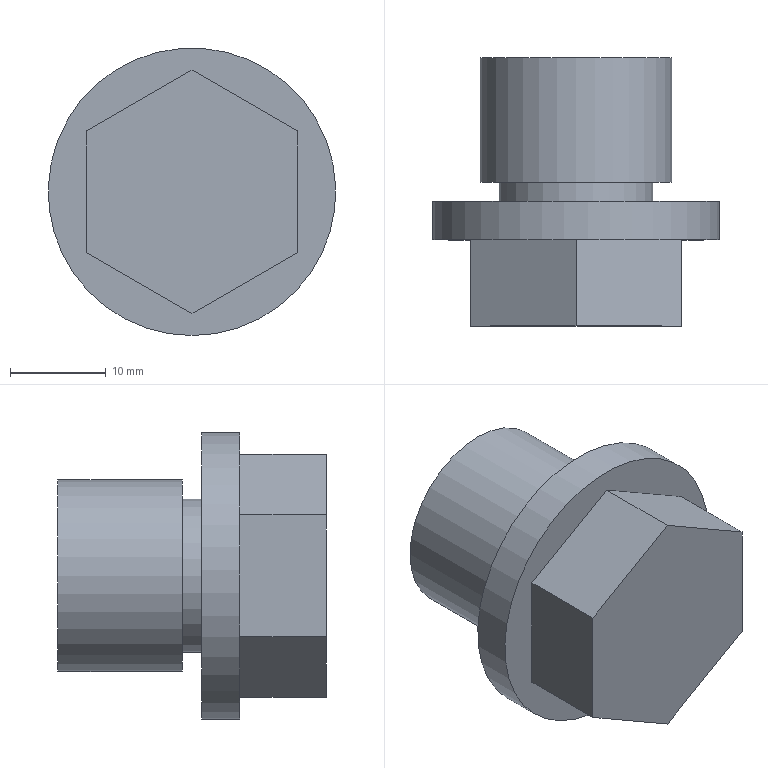Part | NX | features DATUM_CSYS 3, SKETCH 2, EXTRUDE 1, SWP104 1, SYMBOLIC_THREAD 1 | 1 solid | 14 faces | box 30 x 28 x 30 mm | volume 11086 mm3 | plane 11 | cylinder 3 | commonest cylinder face diameters 16 x1 20 x1 30 x1
STEP:
#1=CARTESIAN_POINT('',(-11.,0.,6.351));
#2=VERTEX_POINT('',#1);
#3=CARTESIAN_POINT('',(-11.,0.,-6.351));
#4=VERTEX_POINT('',#3);
#5=CARTESIAN_POINT('',(-11.,0.,6.351));
#6=DIRECTION('',(0.,0.,-1.));
#7=VECTOR('',#6,1000.);
#8=LINE('',#5,#7);
#9=EDGE_CURVE('',#2,#4,#8,.T.);
#10=ORIENTED_EDGE('',*,*,#9,.T.);
#11=CARTESIAN_POINT('',(-11.,-9.,-6.351));
#12=VERTEX_POINT('',#11);
#13=CARTESIAN_POINT('',(-11.,-9.,-6.351));
#14=DIRECTION('',(0.,1.,0.));
#15=VECTOR('',#14,1000.);
#16=LINE('',#13,#15);
#17=EDGE_CURVE('',#12,#4,#16,.T.);
#18=ORIENTED_EDGE('',*,*,#17,.F.);
#19=CARTESIAN_POINT('',(-11.,-9.,6.351));
#20=VERTEX_POINT('',#19);
#21=CARTESIAN_POINT('',(-11.,-9.,6.351));
#22=DIRECTION('',(0.,0.,-1.));
#23=VECTOR('',#22,1000.);
#24=LINE('',#21,#23);
#25=EDGE_CURVE('',#20,#12,#24,.T.);
#26=ORIENTED_EDGE('',*,*,#25,.F.);
#27=CARTESIAN_POINT('',(-11.,-9.,6.351));
#28=DIRECTION('',(0.,1.,0.));
#29=VECTOR('',#28,1000.);
#30=LINE('',#27,#29);
#31=EDGE_CURVE('',#20,#2,#30,.T.);
#32=ORIENTED_EDGE('',*,*,#31,.T.);
#33=EDGE_LOOP('',(#10,#18,#26,#32));
#34=FACE_BOUND('',#33,.T.);
#35=CARTESIAN_POINT('',(-11.,-9.,6.351));
#36=DIRECTION('',(1.,0.,0.));
#37=DIRECTION('',(0.,0.,-1.));
#38=AXIS2_PLACEMENT_3D('',#35,#36,#37);
#39=PLANE('',#38);
#40=ADVANCED_FACE('',(#34),#39,.F.);
#41=CARTESIAN_POINT('',(0.,0.,-12.702));
#42=VERTEX_POINT('',#41);
#43=CARTESIAN_POINT('',(-11.,0.,-6.351));
#44=DIRECTION('',(0.866,0.,-0.5));
#45=VECTOR('',#44,1000.);
#46=LINE('',#43,#45);
#47=EDGE_CURVE('',#4,#42,#46,.T.);
#48=ORIENTED_EDGE('',*,*,#47,.T.);
#49=CARTESIAN_POINT('',(0.,-9.,-12.702));
#50=VERTEX_POINT('',#49);
#51=CARTESIAN_POINT('',(0.,-9.,-12.702));
#52=DIRECTION('',(0.,1.,0.));
#53=VECTOR('',#52,1000.);
#54=LINE('',#51,#53);
#55=EDGE_CURVE('',#50,#42,#54,.T.);
#56=ORIENTED_EDGE('',*,*,#55,.F.);
#57=CARTESIAN_POINT('',(-11.,-9.,-6.351));
#58=DIRECTION('',(0.866,0.,-0.5));
#59=VECTOR('',#58,1000.);
#60=LINE('',#57,#59);
#61=EDGE_CURVE('',#12,#50,#60,.T.);
#62=ORIENTED_EDGE('',*,*,#61,.F.);
#63=ORIENTED_EDGE('',*,*,#17,.T.);
#64=EDGE_LOOP('',(#48,#56,#62,#63));
#65=FACE_BOUND('',#64,.T.);
#66=CARTESIAN_POINT('',(-11.,-9.,-6.351));
#67=DIRECTION('',(0.5,0.,0.866));
#68=DIRECTION('',(0.866,0.,-0.5));
#69=AXIS2_PLACEMENT_3D('',#66,#67,#68);
#70=PLANE('',#69);
#71=ADVANCED_FACE('',(#65),#70,.F.);
#72=CARTESIAN_POINT('',(11.,0.,-6.351));
#73=VERTEX_POINT('',#72);
#74=CARTESIAN_POINT('',(0.,0.,-12.702));
#75=DIRECTION('',(0.866,0.,0.5));
#76=VECTOR('',#75,1000.);
#77=LINE('',#74,#76);
#78=EDGE_CURVE('',#42,#73,#77,.T.);
#79=ORIENTED_EDGE('',*,*,#78,.T.);
#80=CARTESIAN_POINT('',(11.,-9.,-6.351));
#81=VERTEX_POINT('',#80);
#82=CARTESIAN_POINT('',(11.,-9.,-6.351));
#83=DIRECTION('',(0.,1.,0.));
#84=VECTOR('',#83,1000.);
#85=LINE('',#82,#84);
#86=EDGE_CURVE('',#81,#73,#85,.T.);
#87=ORIENTED_EDGE('',*,*,#86,.F.);
#88=CARTESIAN_POINT('',(0.,-9.,-12.702));
#89=DIRECTION('',(0.866,0.,0.5));
#90=VECTOR('',#89,1000.);
#91=LINE('',#88,#90);
#92=EDGE_CURVE('',#50,#81,#91,.T.);
#93=ORIENTED_EDGE('',*,*,#92,.F.);
#94=ORIENTED_EDGE('',*,*,#55,.T.);
#95=EDGE_LOOP('',(#79,#87,#93,#94));
#96=FACE_BOUND('',#95,.T.);
#97=CARTESIAN_POINT('',(0.,-9.,-12.702));
#98=DIRECTION('',(-0.5,0.,0.866));
#99=DIRECTION('',(0.866,0.,0.5));
#100=AXIS2_PLACEMENT_3D('',#97,#98,#99);
#101=PLANE('',#100);
#102=ADVANCED_FACE('',(#96),#101,.F.);
#103=CARTESIAN_POINT('',(11.,0.,6.351));
#104=VERTEX_POINT('',#103);
#105=CARTESIAN_POINT('',(11.,0.,-6.351));
#106=DIRECTION('',(0.,0.,1.));
#107=VECTOR('',#106,1000.);
#108=LINE('',#105,#107);
#109=EDGE_CURVE('',#73,#104,#108,.T.);
#110=ORIENTED_EDGE('',*,*,#109,.T.);
#111=CARTESIAN_POINT('',(11.,-9.,6.351));
#112=VERTEX_POINT('',#111);
#113=CARTESIAN_POINT('',(11.,-9.,6.351));
#114=DIRECTION('',(0.,1.,0.));
#115=VECTOR('',#114,1000.);
#116=LINE('',#113,#115);
#117=EDGE_CURVE('',#112,#104,#116,.T.);
#118=ORIENTED_EDGE('',*,*,#117,.F.);
#119=CARTESIAN_POINT('',(11.,-9.,-6.351));
#120=DIRECTION('',(0.,0.,1.));
#121=VECTOR('',#120,1000.);
#122=LINE('',#119,#121);
#123=EDGE_CURVE('',#81,#112,#122,.T.);
#124=ORIENTED_EDGE('',*,*,#123,.F.);
#125=ORIENTED_EDGE('',*,*,#86,.T.);
#126=EDGE_LOOP('',(#110,#118,#124,#125));
#127=FACE_BOUND('',#126,.T.);
#128=CARTESIAN_POINT('',(11.,-9.,-6.351));
#129=DIRECTION('',(-1.,0.,0.));
#130=DIRECTION('',(0.,0.,1.));
#131=AXIS2_PLACEMENT_3D('',#128,#129,#130);
#132=PLANE('',#131);
#133=ADVANCED_FACE('',(#127),#132,.F.);
#134=CARTESIAN_POINT('',(0.,0.,12.702));
#135=VERTEX_POINT('',#134);
#136=CARTESIAN_POINT('',(11.,0.,6.351));
#137=DIRECTION('',(-0.866,0.,0.5));
#138=VECTOR('',#137,1000.);
#139=LINE('',#136,#138);
#140=EDGE_CURVE('',#104,#135,#139,.T.);
#141=ORIENTED_EDGE('',*,*,#140,.T.);
#142=CARTESIAN_POINT('',(0.,-9.,12.702));
#143=VERTEX_POINT('',#142);
#144=CARTESIAN_POINT('',(0.,-9.,12.702));
#145=DIRECTION('',(0.,1.,0.));
#146=VECTOR('',#145,1000.);
#147=LINE('',#144,#146);
#148=EDGE_CURVE('',#143,#135,#147,.T.);
#149=ORIENTED_EDGE('',*,*,#148,.F.);
#150=CARTESIAN_POINT('',(11.,-9.,6.351));
#151=DIRECTION('',(-0.866,0.,0.5));
#152=VECTOR('',#151,1000.);
#153=LINE('',#150,#152);
#154=EDGE_CURVE('',#112,#143,#153,.T.);
#155=ORIENTED_EDGE('',*,*,#154,.F.);
#156=ORIENTED_EDGE('',*,*,#117,.T.);
#157=EDGE_LOOP('',(#141,#149,#155,#156));
#158=FACE_BOUND('',#157,.T.);
#159=CARTESIAN_POINT('',(11.,-9.,6.351));
#160=DIRECTION('',(-0.5,0.,-0.866));
#161=DIRECTION('',(-0.866,0.,0.5));
#162=AXIS2_PLACEMENT_3D('',#159,#160,#161);
#163=PLANE('',#162);
#164=ADVANCED_FACE('',(#158),#163,.F.);
#165=CARTESIAN_POINT('',(0.,0.,12.702));
#166=DIRECTION('',(-0.866,0.,-0.5));
#167=VECTOR('',#166,1000.);
#168=LINE('',#165,#167);
#169=EDGE_CURVE('',#135,#2,#168,.T.);
#170=ORIENTED_EDGE('',*,*,#169,.T.);
#171=ORIENTED_EDGE('',*,*,#31,.F.);
#172=CARTESIAN_POINT('',(0.,-9.,12.702));
#173=DIRECTION('',(-0.866,0.,-0.5));
#174=VECTOR('',#173,1000.);
#175=LINE('',#172,#174);
#176=EDGE_CURVE('',#143,#20,#175,.T.);
#177=ORIENTED_EDGE('',*,*,#176,.F.);
#178=ORIENTED_EDGE('',*,*,#148,.T.);
#179=EDGE_LOOP('',(#170,#171,#177,#178));
#180=FACE_BOUND('',#179,.T.);
#181=CARTESIAN_POINT('',(0.,-9.,12.702));
#182=DIRECTION('',(0.5,0.,-0.866));
#183=DIRECTION('',(-0.866,0.,-0.5));
#184=AXIS2_PLACEMENT_3D('',#181,#182,#183);
#185=PLANE('',#184);
#186=ADVANCED_FACE('',(#180),#185,.F.);
#187=ORIENTED_EDGE('',*,*,#25,.T.);
#188=ORIENTED_EDGE('',*,*,#61,.T.);
#189=ORIENTED_EDGE('',*,*,#92,.T.);
#190=ORIENTED_EDGE('',*,*,#123,.T.);
#191=ORIENTED_EDGE('',*,*,#154,.T.);
#192=ORIENTED_EDGE('',*,*,#176,.T.);
#193=EDGE_LOOP('',(#187,#188,#189,#190,#191,#192));
#194=FACE_BOUND('',#193,.T.);
#195=CARTESIAN_POINT('',(0.,-9.,0.));
#196=DIRECTION('',(0.,-1.,0.));
#197=DIRECTION('',(0.,0.,-1.));
#198=AXIS2_PLACEMENT_3D('',#195,#196,#197);
#199=PLANE('',#198);
#200=ADVANCED_FACE('',(#194),#199,.T.);
#201=ORIENTED_EDGE('',*,*,#9,.F.);
#202=ORIENTED_EDGE('',*,*,#169,.F.);
#203=ORIENTED_EDGE('',*,*,#140,.F.);
#204=ORIENTED_EDGE('',*,*,#109,.F.);
#205=ORIENTED_EDGE('',*,*,#78,.F.);
#206=ORIENTED_EDGE('',*,*,#47,.F.);
#207=EDGE_LOOP('',(#201,#202,#203,#204,#205,#206));
#208=FACE_BOUND('',#207,.T.);
#209=CARTESIAN_POINT('',(0.,0.,-15.));
#210=VERTEX_POINT('',#209);
#211=CARTESIAN_POINT('',(0.,0.,0.));
#212=DIRECTION('',(0.,-1.,0.));
#213=DIRECTION('',(0.,0.,-1.));
#214=AXIS2_PLACEMENT_3D('',#211,#212,#213);
#215=CIRCLE('',#214,15.);
#216=EDGE_CURVE('',#210,#210,#215,.T.);
#217=ORIENTED_EDGE('',*,*,#216,.T.);
#218=EDGE_LOOP('',(#217));
#219=FACE_BOUND('',#218,.T.);
#220=CARTESIAN_POINT('',(0.,0.,15.));
#221=DIRECTION('',(0.,1.,0.));
#222=DIRECTION('',(0.,0.,1.));
#223=AXIS2_PLACEMENT_3D('',#220,#221,#222);
#224=PLANE('',#223);
#225=ADVANCED_FACE('',(#208,#219),#224,.F.);
#226=CARTESIAN_POINT('',(0.,19.,-10.));
#227=VERTEX_POINT('',#226);
#228=CARTESIAN_POINT('',(0.,19.,0.));
#229=DIRECTION('',(0.,-1.,0.));
#230=DIRECTION('',(0.,0.,-1.));
#231=AXIS2_PLACEMENT_3D('',#228,#229,#230);
#232=CIRCLE('',#231,10.);
#233=EDGE_CURVE('',#227,#227,#232,.T.);
#234=ORIENTED_EDGE('',*,*,#233,.F.);
#235=EDGE_LOOP('',(#234));
#236=FACE_BOUND('',#235,.T.);
#237=CARTESIAN_POINT('',(0.,19.,0.));
#238=DIRECTION('',(0.,-1.,0.));
#239=DIRECTION('',(0.,0.,-1.));
#240=AXIS2_PLACEMENT_3D('',#237,#238,#239);
#241=PLANE('',#240);
#242=ADVANCED_FACE('',(#236),#241,.F.);
#243=CARTESIAN_POINT('',(0.,6.,-10.));
#244=VERTEX_POINT('',#243);
#245=CARTESIAN_POINT('',(0.,6.,0.));
#246=DIRECTION('',(0.,-1.,0.));
#247=DIRECTION('',(0.,0.,-1.));
#248=AXIS2_PLACEMENT_3D('',#245,#246,#247);
#249=CIRCLE('',#248,10.);
#250=EDGE_CURVE('',#244,#244,#249,.T.);
#251=ORIENTED_EDGE('',*,*,#250,.F.);
#252=EDGE_LOOP('',(#251));
#253=FACE_BOUND('',#252,.T.);
#254=ORIENTED_EDGE('',*,*,#233,.T.);
#255=EDGE_LOOP('',(#254));
#256=FACE_BOUND('',#255,.T.);
#257=CARTESIAN_POINT('',(0.,19.,0.));
#258=DIRECTION('',(0.,-1.,0.));
#259=DIRECTION('',(0.,0.,-1.));
#260=AXIS2_PLACEMENT_3D('',#257,#258,#259);
#261=CYLINDRICAL_SURFACE('',#260,10.);
#262=ADVANCED_FACE('',(#253,#256),#261,.T.);
#263=CARTESIAN_POINT('',(0.,6.,-8.));
#264=VERTEX_POINT('',#263);
#265=CARTESIAN_POINT('',(0.,6.,0.));
#266=DIRECTION('',(0.,-1.,0.));
#267=DIRECTION('',(0.,0.,-1.));
#268=AXIS2_PLACEMENT_3D('',#265,#266,#267);
#269=CIRCLE('',#268,8.);
#270=EDGE_CURVE('',#264,#264,#269,.T.);
#271=ORIENTED_EDGE('',*,*,#270,.F.);
#272=EDGE_LOOP('',(#271));
#273=FACE_BOUND('',#272,.T.);
#274=ORIENTED_EDGE('',*,*,#250,.T.);
#275=EDGE_LOOP('',(#274));
#276=FACE_BOUND('',#275,.T.);
#277=CARTESIAN_POINT('',(0.,6.,10.));
#278=DIRECTION('',(0.,1.,0.));
#279=DIRECTION('',(0.,0.,1.));
#280=AXIS2_PLACEMENT_3D('',#277,#278,#279);
#281=PLANE('',#280);
#282=ADVANCED_FACE('',(#273,#276),#281,.F.);
#283=CARTESIAN_POINT('',(0.,4.,-8.));
#284=VERTEX_POINT('',#283);
#285=CARTESIAN_POINT('',(0.,4.,0.));
#286=DIRECTION('',(0.,-1.,0.));
#287=DIRECTION('',(0.,0.,-1.));
#288=AXIS2_PLACEMENT_3D('',#285,#286,#287);
#289=CIRCLE('',#288,8.);
#290=EDGE_CURVE('',#284,#284,#289,.T.);
#291=ORIENTED_EDGE('',*,*,#290,.F.);
#292=EDGE_LOOP('',(#291));
#293=FACE_BOUND('',#292,.T.);
#294=ORIENTED_EDGE('',*,*,#270,.T.);
#295=EDGE_LOOP('',(#294));
#296=FACE_BOUND('',#295,.T.);
#297=CARTESIAN_POINT('',(0.,19.,0.));
#298=DIRECTION('',(0.,-1.,0.));
#299=DIRECTION('',(0.,0.,-1.));
#300=AXIS2_PLACEMENT_3D('',#297,#298,#299);
#301=CYLINDRICAL_SURFACE('',#300,8.);
#302=ADVANCED_FACE('',(#293,#296),#301,.T.);
#303=CARTESIAN_POINT('',(0.,4.,-15.));
#304=VERTEX_POINT('',#303);
#305=CARTESIAN_POINT('',(0.,4.,0.));
#306=DIRECTION('',(0.,-1.,0.));
#307=DIRECTION('',(0.,0.,-1.));
#308=AXIS2_PLACEMENT_3D('',#305,#306,#307);
#309=CIRCLE('',#308,15.);
#310=EDGE_CURVE('',#304,#304,#309,.T.);
#311=ORIENTED_EDGE('',*,*,#310,.F.);
#312=EDGE_LOOP('',(#311));
#313=FACE_BOUND('',#312,.T.);
#314=ORIENTED_EDGE('',*,*,#290,.T.);
#315=EDGE_LOOP('',(#314));
#316=FACE_BOUND('',#315,.T.);
#317=CARTESIAN_POINT('',(0.,4.,8.));
#318=DIRECTION('',(0.,-1.,0.));
#319=DIRECTION('',(0.,0.,-1.));
#320=AXIS2_PLACEMENT_3D('',#317,#318,#319);
#321=PLANE('',#320);
#322=ADVANCED_FACE('',(#313,#316),#321,.F.);
#323=ORIENTED_EDGE('',*,*,#216,.F.);
#324=EDGE_LOOP('',(#323));
#325=FACE_BOUND('',#324,.T.);
#326=ORIENTED_EDGE('',*,*,#310,.T.);
#327=EDGE_LOOP('',(#326));
#328=FACE_BOUND('',#327,.T.);
#329=CARTESIAN_POINT('',(0.,19.,0.));
#330=DIRECTION('',(0.,-1.,0.));
#331=DIRECTION('',(0.,0.,-1.));
#332=AXIS2_PLACEMENT_3D('',#329,#330,#331);
#333=CYLINDRICAL_SURFACE('',#332,15.);
#334=ADVANCED_FACE('',(#325,#328),#333,.T.);
#335=CLOSED_SHELL('',(#40,#71,#102,#133,#164,#186,#200,#225,#242,#262,#282,#302,#322,#334));
#336=MANIFOLD_SOLID_BREP('',#335);
#337=(LENGTH_UNIT()NAMED_UNIT(*)SI_UNIT(.MILLI.,.METRE.));
#338=UNCERTAINTY_MEASURE_WITH_UNIT(LENGTH_MEASURE(0.00001),#337,'','');
#339=(NAMED_UNIT(*)PLANE_ANGLE_UNIT()SI_UNIT($,.RADIAN.));
#340=(NAMED_UNIT(*)SI_UNIT($,.STERADIAN.)SOLID_ANGLE_UNIT());
#341=(GEOMETRIC_REPRESENTATION_CONTEXT(3)GLOBAL_UNCERTAINTY_ASSIGNED_CONTEXT((#338))GLOBAL_UNIT_ASSIGNED_CONTEXT((#337,#339,#340))REPRESENTATION_CONTEXT('',''));
#342=ADVANCED_BREP_SHAPE_REPRESENTATION('',(#336),#341);